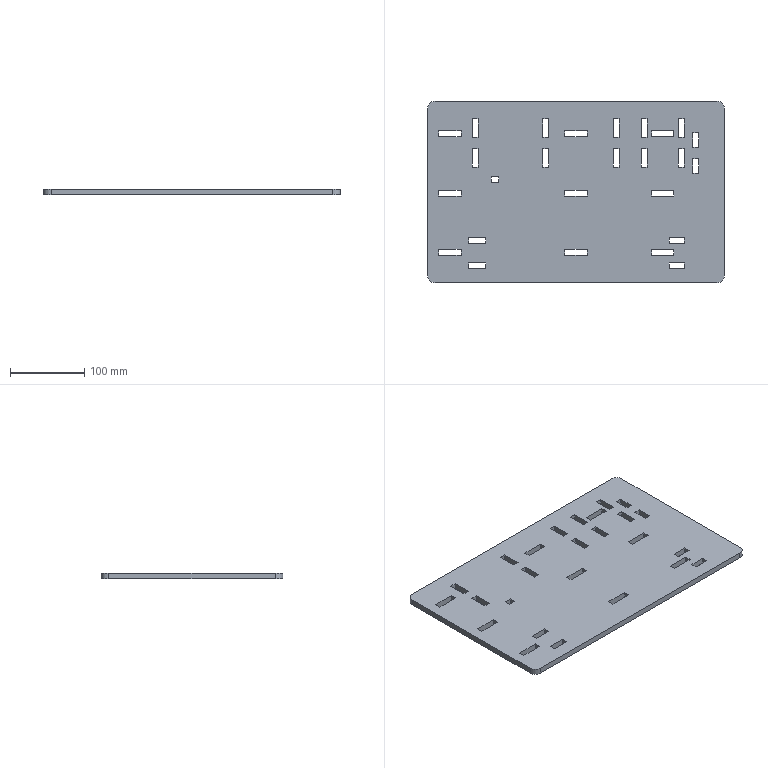Part | SolidWorks | features FlatPattern 1, SMBaseFlange 1, SheetMetal 1 | 1 solid | 114 faces | box 400 x 245 x 8 mm | volume 741201 mm3 | plane 110 | cylinder 4 | commonest cylinder face diameters 20 x4